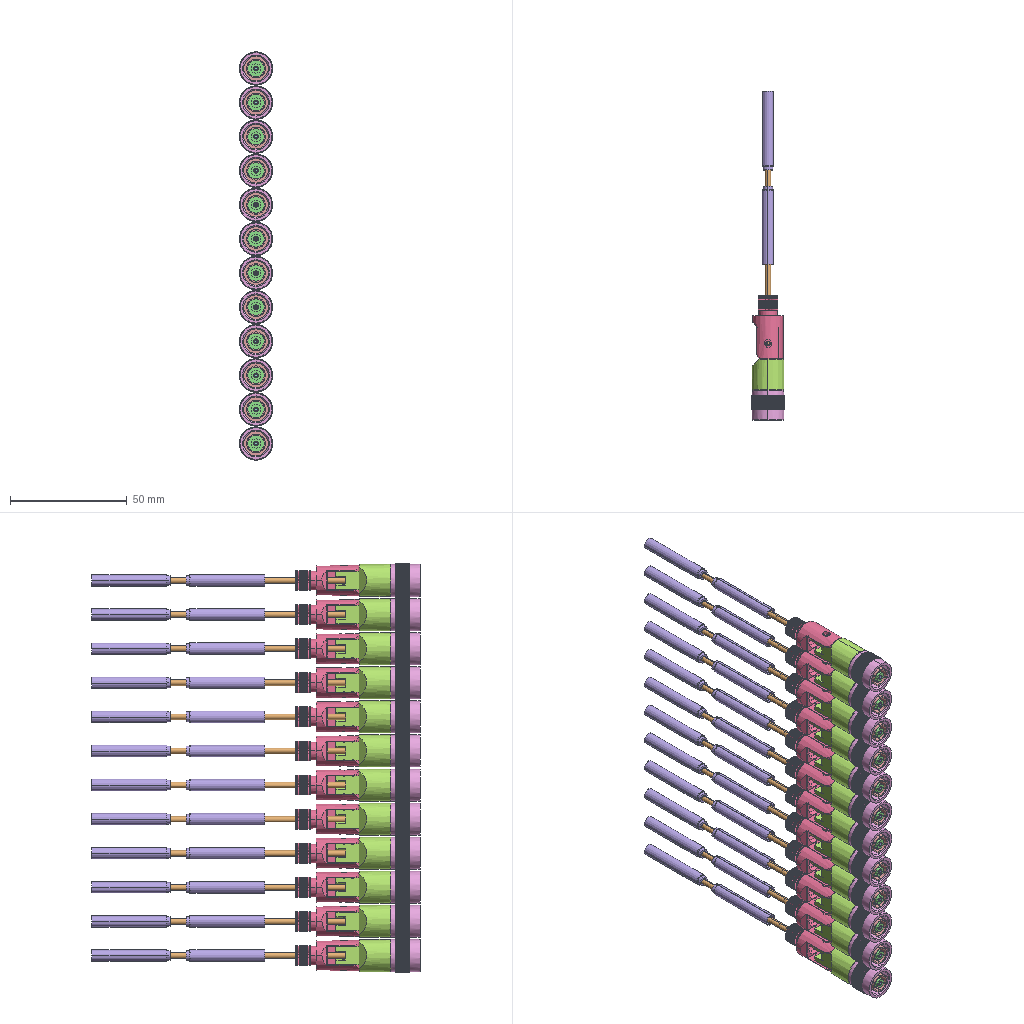Assembly | SolidWorks | 10 different items | 121 placed | box 14 x 141 x 175 mm
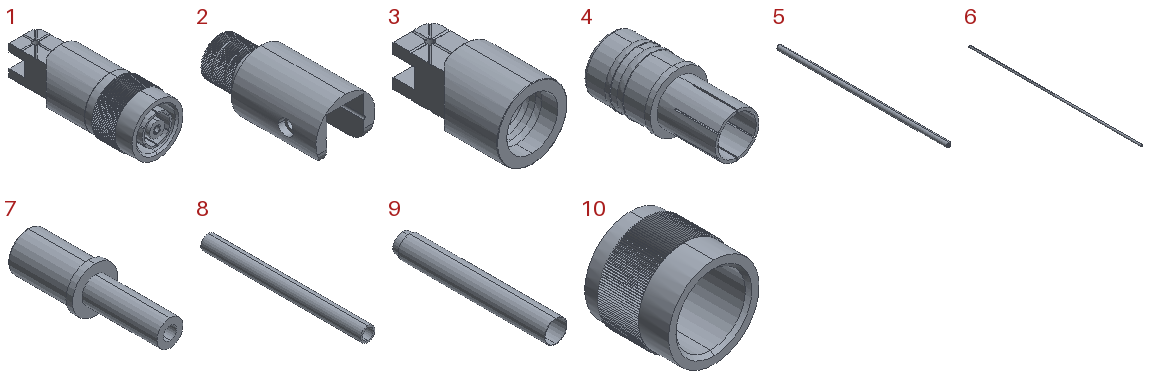Parts list (item | name | quantity | size | volume | features):
1 | (subassembly) | x1 | 14.217 x 36.1 x 14.22 mm | 3487 mm3 | -
2 | - | x12 | 12.92 x 27.3 x 12.92 mm | 1231 mm3 | features ICE 6, RevCut 2, Chamfer 1, Revolution 1
3 | - | x12 | 13.72 x 23.4 x 13.72 mm | 1526 mm3 | features ICE 7, Fillet 2, MirrorPattern 1, Revolution 1
4 | - | x12 | 10.5 x 23 x 10.5 mm | 736.39 mm3 | features CirPattern 1, Fillet 1, ICE 1, Revolution 1
5 | - | x12 | 2.4 x 85 x 2.4 mm | 317.772 mm3 | features Revolution 1
6 | - | x12 | 1 x 90 x 1 mm | 70.686 mm3 | features Revolution 1
7 | - | x12 | 7 x 22 x 7 mm | 384.292 mm3 | features Fillet 1, Revolution 1
8 | - | x12 | 2 x 22 x 2 mm | 30.238 mm3 | features Revolution 1
9 | - | x24 | 4.9 x 33.507 x 4.9 mm | 63.209 mm3 | features Revolution 1
10 | - | x12 | 14.217 x 12.7 x 14.22 mm | 809.778 mm3 | features Chamfer 1, ICE 1, Revolution 1
Mates (type | each side: item.copy, entity, surface, feature):
Concentric | 4.1 face cylinder Revolve1 | 3.1 face cylinder Revolve1
DistanceDim | 4.1 face plane Revolve1 | 3.1 face plane Revolve1
Coincident | 4.1 face plane Revolve1 | 10.1 face plane Revolve1
Coordinate | 4.1 select_type:25 | assembly select_type:11
Concentric | 4.1 face cylinder Revolve1 | 10.1 face cylinder Revolve1
Concentric | 8.1 face cylinder Revolve1 | 3.1 face cylinder Cut-Extrude2
Coincident | 4.1 face plane Revolve1 | 8.1 face plane Revolve1
Concentric | 8.1 face cylinder Revolve1 | 6.1 face cylinder Revolve1
DistanceDim | 8.1 face plane Revolve1 | 6.1 face plane Revolve1
Concentric | 6.1 face cylinder Revolve1 | 5.1 face cylinder Revolve1
DistanceDim | 5.1 face plane Revolve1 | 6.1 face plane Revolve1
Concentric | 6.1 face cylinder Revolve1 | 9.1 face cylinder Revolve1
Concentric | 5.1 face cylinder Revolve1 | 9.2 face cylinder Revolve1
DistanceDim | 9.2 face plane Revolve1 | 9.1 face plane Revolve1
Concentric | 4.1 face cylinder Revolve1 | 7.1 face cylinder Revolve1
Coincident | 4.1 edge | 7.1 face plane Revolve1
Coincident | 5.1 face plane Revolve1 | 9.1 face plane Revolve1
Coincident | 2.1 plane | assembly plane